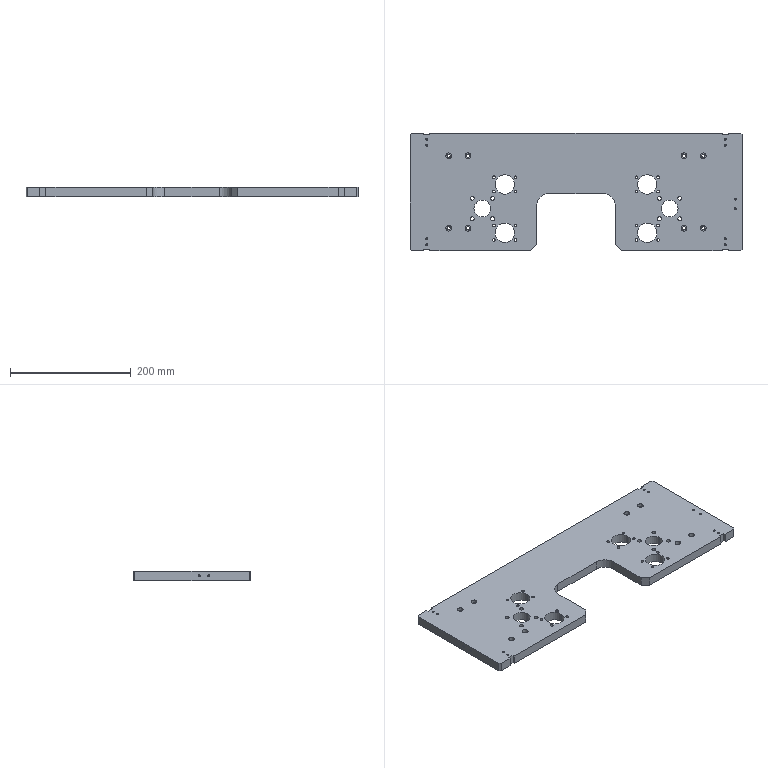Part | STEP file | 227H056239 Base | 1 solid | 229 faces | box 550 x 195 x 15 mm | volume 1337407 mm3 | cylinder 146 | plane 49 | cone 34 | commonest cylinder face diameters 4.2 x32 3.3 x26 5.5 x16 6.6 x16 9.5 x16 11 x16